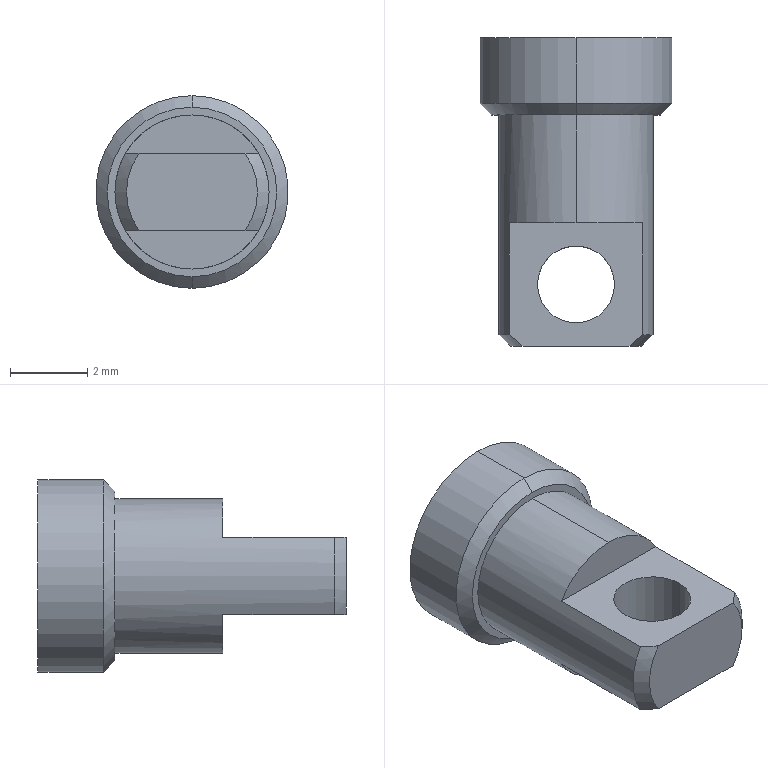Part | SolidWorks | features ICE 3, Chamfer 1, Extrusion 1, HoleWzd 1 | 1 solid | 21 faces | box 5 x 8 x 5 mm | volume 68.475 mm3 | cylinder 8 | plane 7 | cone 6 | commonest cylinder face diameters 2 x2 2.5 x2 4 x2 5 x2
STEP:
#1=CARTESIAN_POINT('',(1.,1.6,-1.));
#2=VERTEX_POINT('',#1);
#3=CARTESIAN_POINT('',(-1.,1.6,-1.));
#4=VERTEX_POINT('',#3);
#5=CARTESIAN_POINT('',(0.,1.6,-1.));
#6=DIRECTION('',(0.,0.,-1.));
#7=DIRECTION('',(1.,0.,0.));
#8=AXIS2_PLACEMENT_3D('',#5,#6,#7);
#9=CIRCLE('',#8,1.);
#10=EDGE_CURVE('',#2,#4,#9,.T.);
#11=ORIENTED_EDGE('',*,*,#10,.T.);
#12=CARTESIAN_POINT('',(-1.,1.6,1.));
#13=VERTEX_POINT('',#12);
#14=CARTESIAN_POINT('',(-1.,1.6,-5.));
#15=DIRECTION('',(0.,0.,1.));
#16=VECTOR('',#15,1000.);
#17=LINE('',#14,#16);
#18=EDGE_CURVE('',#4,#13,#17,.T.);
#19=ORIENTED_EDGE('',*,*,#18,.T.);
#20=CARTESIAN_POINT('',(1.,1.6,1.));
#21=VERTEX_POINT('',#20);
#22=CARTESIAN_POINT('',(0.,1.6,1.));
#23=DIRECTION('',(0.,0.,1.));
#24=DIRECTION('',(-1.,0.,0.));
#25=AXIS2_PLACEMENT_3D('',#22,#23,#24);
#26=CIRCLE('',#25,1.);
#27=EDGE_CURVE('',#13,#21,#26,.T.);
#28=ORIENTED_EDGE('',*,*,#27,.T.);
#29=CARTESIAN_POINT('',(1.,1.6,-5.));
#30=DIRECTION('',(0.,0.,1.));
#31=VECTOR('',#30,1000.);
#32=LINE('',#29,#31);
#33=EDGE_CURVE('',#2,#21,#32,.T.);
#34=ORIENTED_EDGE('',*,*,#33,.F.);
#35=EDGE_LOOP('',(#11,#19,#28,#34));
#36=FACE_OUTER_BOUND('',#35,.T.);
#37=CARTESIAN_POINT('',(0.,1.6,-5.));
#38=DIRECTION('',(0.,0.,1.));
#39=DIRECTION('',(1.,0.,0.));
#40=AXIS2_PLACEMENT_3D('',#37,#38,#39);
#41=CYLINDRICAL_SURFACE('',#40,1.);
#42=ADVANCED_FACE('',(#36),#41,.F.);
#43=CARTESIAN_POINT('',(0.,6.,-2.2));
#44=VERTEX_POINT('',#43);
#45=CARTESIAN_POINT('',(0.,6.,2.2));
#46=VERTEX_POINT('',#45);
#47=CARTESIAN_POINT('',(0.,6.,0.));
#48=DIRECTION('',(0.,-1.,0.));
#49=DIRECTION('',(0.,0.,1.));
#50=AXIS2_PLACEMENT_3D('',#47,#48,#49);
#51=CIRCLE('',#50,2.2);
#52=EDGE_CURVE('',#44,#46,#51,.T.);
#53=ORIENTED_EDGE('',*,*,#52,.F.);
#54=CARTESIAN_POINT('',(0.,6.3,-2.5));
#55=VERTEX_POINT('',#54);
#56=CARTESIAN_POINT('',(0.,6.3,-2.5));
#57=DIRECTION('',(0.,0.7071,-0.7071));
#58=VECTOR('',#57,1000.);
#59=LINE('',#56,#58);
#60=EDGE_CURVE('',#44,#55,#59,.T.);
#61=ORIENTED_EDGE('',*,*,#60,.T.);
#62=CARTESIAN_POINT('',(0.,6.3,2.5));
#63=VERTEX_POINT('',#62);
#64=CARTESIAN_POINT('',(0.,6.3,0.));
#65=DIRECTION('',(0.,1.,0.));
#66=DIRECTION('',(0.,0.,1.));
#67=AXIS2_PLACEMENT_3D('',#64,#65,#66);
#68=CIRCLE('',#67,2.5);
#69=EDGE_CURVE('',#63,#55,#68,.T.);
#70=ORIENTED_EDGE('',*,*,#69,.F.);
#71=CARTESIAN_POINT('',(0.,6.3,2.5));
#72=DIRECTION('',(0.,0.7071,0.7071));
#73=VECTOR('',#72,1000.);
#74=LINE('',#71,#73);
#75=EDGE_CURVE('',#46,#63,#74,.T.);
#76=ORIENTED_EDGE('',*,*,#75,.F.);
#77=EDGE_LOOP('',(#53,#61,#70,#76));
#78=FACE_OUTER_BOUND('',#77,.T.);
#79=CARTESIAN_POINT('',(0.,6.3,0.));
#80=DIRECTION('',(0.,1.,0.));
#81=DIRECTION('',(0.,0.,1.));
#82=AXIS2_PLACEMENT_3D('',#79,#80,#81);
#83=CONICAL_SURFACE('',#82,2.5,0.7854);
#84=ADVANCED_FACE('',(#78),#83,.T.);
#85=CARTESIAN_POINT('',(0.,3.5,-1.25));
#86=VERTEX_POINT('',#85);
#87=CARTESIAN_POINT('',(0.,3.5,1.25));
#88=VERTEX_POINT('',#87);
#89=CARTESIAN_POINT('',(0.,3.5,0.));
#90=DIRECTION('',(0.,1.,0.));
#91=DIRECTION('',(0.,0.,1.));
#92=AXIS2_PLACEMENT_3D('',#89,#90,#91);
#93=CIRCLE('',#92,1.25);
#94=EDGE_CURVE('',#86,#88,#93,.T.);
#95=ORIENTED_EDGE('',*,*,#94,.F.);
#96=CARTESIAN_POINT('',(0.,8.,-1.25));
#97=VERTEX_POINT('',#96);
#98=CARTESIAN_POINT('',(0.,8.,-1.25));
#99=DIRECTION('',(0.,1.,0.));
#100=VECTOR('',#99,1000.);
#101=LINE('',#98,#100);
#102=EDGE_CURVE('',#86,#97,#101,.T.);
#103=ORIENTED_EDGE('',*,*,#102,.T.);
#104=CARTESIAN_POINT('',(0.,8.,1.25));
#105=VERTEX_POINT('',#104);
#106=CARTESIAN_POINT('',(0.,8.,0.));
#107=DIRECTION('',(0.,1.,0.));
#108=DIRECTION('',(0.,0.,1.));
#109=AXIS2_PLACEMENT_3D('',#106,#107,#108);
#110=CIRCLE('',#109,1.25);
#111=EDGE_CURVE('',#97,#105,#110,.T.);
#112=ORIENTED_EDGE('',*,*,#111,.T.);
#113=CARTESIAN_POINT('',(0.,8.,1.25));
#114=DIRECTION('',(0.,1.,0.));
#115=VECTOR('',#114,1000.);
#116=LINE('',#113,#115);
#117=EDGE_CURVE('',#88,#105,#116,.T.);
#118=ORIENTED_EDGE('',*,*,#117,.F.);
#119=EDGE_LOOP('',(#95,#103,#112,#118));
#120=FACE_OUTER_BOUND('',#119,.T.);
#121=CARTESIAN_POINT('',(0.,8.,0.));
#122=DIRECTION('',(0.,1.,0.));
#123=DIRECTION('',(0.,0.,1.));
#124=AXIS2_PLACEMENT_3D('',#121,#122,#123);
#125=CYLINDRICAL_SURFACE('',#124,1.25);
#126=ADVANCED_FACE('',(#120),#125,.F.);
#127=CARTESIAN_POINT('',(0.,2.749,0.));
#128=VERTEX_POINT('',#127);
#129=CARTESIAN_POINT('',(0.,3.5,1.25));
#130=DIRECTION('',(0.,0.515,0.8572));
#131=VECTOR('',#130,1000.);
#132=LINE('',#129,#131);
#133=EDGE_CURVE('',#128,#88,#132,.T.);
#134=ORIENTED_EDGE('',*,*,#133,.F.);
#135=CARTESIAN_POINT('',(0.,3.5,-1.25));
#136=DIRECTION('',(0.,0.515,-0.8572));
#137=VECTOR('',#136,1000.);
#138=LINE('',#135,#137);
#139=EDGE_CURVE('',#128,#86,#138,.T.);
#140=ORIENTED_EDGE('',*,*,#139,.T.);
#141=ORIENTED_EDGE('',*,*,#94,.T.);
#142=EDGE_LOOP('',(#134,#140,#141));
#143=FACE_OUTER_BOUND('',#142,.T.);
#144=CARTESIAN_POINT('',(0.,3.5,0.));
#145=DIRECTION('',(0.,1.,0.));
#146=DIRECTION('',(0.,0.,1.));
#147=AXIS2_PLACEMENT_3D('',#144,#145,#146);
#148=CONICAL_SURFACE('',#147,1.25,1.03);
#149=ADVANCED_FACE('',(#143),#148,.F.);
#150=CARTESIAN_POINT('',(0.,8.,2.5));
#151=VERTEX_POINT('',#150);
#152=CARTESIAN_POINT('',(0.,8.,-2.5));
#153=VERTEX_POINT('',#152);
#154=CARTESIAN_POINT('',(0.,8.,0.));
#155=DIRECTION('',(0.,1.,0.));
#156=DIRECTION('',(0.,0.,1.));
#157=AXIS2_PLACEMENT_3D('',#154,#155,#156);
#158=CIRCLE('',#157,2.5);
#159=EDGE_CURVE('',#151,#153,#158,.T.);
#160=ORIENTED_EDGE('',*,*,#159,.F.);
#161=CARTESIAN_POINT('',(0.,8.,2.5));
#162=DIRECTION('',(0.,-1.,0.));
#163=VECTOR('',#162,1000.);
#164=LINE('',#161,#163);
#165=EDGE_CURVE('',#151,#63,#164,.T.);
#166=ORIENTED_EDGE('',*,*,#165,.T.);
#167=ORIENTED_EDGE('',*,*,#69,.T.);
#168=CARTESIAN_POINT('',(0.,8.,-2.5));
#169=DIRECTION('',(0.,-1.,0.));
#170=VECTOR('',#169,1000.);
#171=LINE('',#168,#170);
#172=EDGE_CURVE('',#153,#55,#171,.T.);
#173=ORIENTED_EDGE('',*,*,#172,.F.);
#174=EDGE_LOOP('',(#160,#166,#167,#173));
#175=FACE_OUTER_BOUND('',#174,.T.);
#176=CARTESIAN_POINT('',(0.,8.,0.));
#177=DIRECTION('',(0.,-1.,0.));
#178=DIRECTION('',(0.,0.,-1.));
#179=AXIS2_PLACEMENT_3D('',#176,#177,#178);
#180=CYLINDRICAL_SURFACE('',#179,2.5);
#181=ADVANCED_FACE('',(#175),#180,.T.);
#182=CARTESIAN_POINT('',(0.,6.,2.));
#183=VERTEX_POINT('',#182);
#184=CARTESIAN_POINT('',(0.,6.,-2.));
#185=VERTEX_POINT('',#184);
#186=CARTESIAN_POINT('',(0.,6.,0.));
#187=DIRECTION('',(0.,1.,0.));
#188=DIRECTION('',(0.,0.,1.));
#189=AXIS2_PLACEMENT_3D('',#186,#187,#188);
#190=CIRCLE('',#189,2.);
#191=EDGE_CURVE('',#183,#185,#190,.T.);
#192=ORIENTED_EDGE('',*,*,#191,.F.);
#193=CARTESIAN_POINT('',(0.,3.2,2.));
#194=VERTEX_POINT('',#193);
#195=CARTESIAN_POINT('',(0.,6.,2.));
#196=DIRECTION('',(0.,-1.,0.));
#197=VECTOR('',#196,1000.);
#198=LINE('',#195,#197);
#199=EDGE_CURVE('',#183,#194,#198,.T.);
#200=ORIENTED_EDGE('',*,*,#199,.T.);
#201=CARTESIAN_POINT('',(1.732,3.2,1.));
#202=VERTEX_POINT('',#201);
#203=CARTESIAN_POINT('',(0.,3.2,0.));
#204=DIRECTION('',(0.,1.,0.));
#205=DIRECTION('',(0.,0.,1.));
#206=AXIS2_PLACEMENT_3D('',#203,#204,#205);
#207=CIRCLE('',#206,2.);
#208=EDGE_CURVE('',#194,#202,#207,.T.);
#209=ORIENTED_EDGE('',*,*,#208,.T.);
#210=CARTESIAN_POINT('',(1.732,0.3,1.));
#211=VERTEX_POINT('',#210);
#212=CARTESIAN_POINT('',(1.732,6.,1.));
#213=DIRECTION('',(0.,-1.,0.));
#214=VECTOR('',#213,1000.);
#215=LINE('',#212,#214);
#216=EDGE_CURVE('',#202,#211,#215,.T.);
#217=ORIENTED_EDGE('',*,*,#216,.T.);
#218=CARTESIAN_POINT('',(1.732,0.3,-1.));
#219=VERTEX_POINT('',#218);
#220=CARTESIAN_POINT('',(0.,0.3,0.));
#221=DIRECTION('',(0.,1.,0.));
#222=DIRECTION('',(0.,0.,1.));
#223=AXIS2_PLACEMENT_3D('',#220,#221,#222);
#224=CIRCLE('',#223,2.);
#225=EDGE_CURVE('',#211,#219,#224,.T.);
#226=ORIENTED_EDGE('',*,*,#225,.T.);
#227=CARTESIAN_POINT('',(1.732,3.2,-1.));
#228=VERTEX_POINT('',#227);
#229=CARTESIAN_POINT('',(1.732,6.,-1.));
#230=DIRECTION('',(0.,1.,0.));
#231=VECTOR('',#230,1000.);
#232=LINE('',#229,#231);
#233=EDGE_CURVE('',#219,#228,#232,.T.);
#234=ORIENTED_EDGE('',*,*,#233,.T.);
#235=CARTESIAN_POINT('',(0.,3.2,-2.));
#236=VERTEX_POINT('',#235);
#237=CARTESIAN_POINT('',(0.,3.2,0.));
#238=DIRECTION('',(0.,1.,0.));
#239=DIRECTION('',(0.,0.,1.));
#240=AXIS2_PLACEMENT_3D('',#237,#238,#239);
#241=CIRCLE('',#240,2.);
#242=EDGE_CURVE('',#228,#236,#241,.T.);
#243=ORIENTED_EDGE('',*,*,#242,.T.);
#244=CARTESIAN_POINT('',(0.,6.,-2.));
#245=DIRECTION('',(0.,-1.,0.));
#246=VECTOR('',#245,1000.);
#247=LINE('',#244,#246);
#248=EDGE_CURVE('',#185,#236,#247,.T.);
#249=ORIENTED_EDGE('',*,*,#248,.F.);
#250=EDGE_LOOP('',(#192,#200,#209,#217,#226,#234,#243,#249));
#251=FACE_OUTER_BOUND('',#250,.T.);
#252=CARTESIAN_POINT('',(0.,6.,0.));
#253=DIRECTION('',(0.,-1.,0.));
#254=DIRECTION('',(0.,0.,-1.));
#255=AXIS2_PLACEMENT_3D('',#252,#253,#254);
#256=CYLINDRICAL_SURFACE('',#255,2.);
#257=ADVANCED_FACE('',(#251),#256,.T.);
#258=CARTESIAN_POINT('',(-1.732,0.3,1.));
#259=VERTEX_POINT('',#258);
#260=CARTESIAN_POINT('',(-1.375,0.,1.));
#261=VERTEX_POINT('',#260);
#262=CARTESIAN_POINT('',(-1.732,0.3,1.));
#263=CARTESIAN_POINT('',(-1.615,0.1982,1.));
#264=CARTESIAN_POINT('',(-1.496,0.09775,1.));
#265=CARTESIAN_POINT('',(-1.375,0.,1.));
#266=B_SPLINE_CURVE_WITH_KNOTS('',3,(#262,#263,#264,#265),.UNSPECIFIED.,.F.,.F.,(4,4),(0.003514,0.00398),.UNSPECIFIED.);
#267=EDGE_CURVE('',#259,#261,#266,.T.);
#268=ORIENTED_EDGE('',*,*,#267,.F.);
#269=CARTESIAN_POINT('',(-1.732,0.3,-1.));
#270=VERTEX_POINT('',#269);
#271=CARTESIAN_POINT('',(0.,0.3,0.));
#272=DIRECTION('',(0.,1.,0.));
#273=DIRECTION('',(0.,0.,1.));
#274=AXIS2_PLACEMENT_3D('',#271,#272,#273);
#275=CIRCLE('',#274,2.);
#276=EDGE_CURVE('',#270,#259,#275,.T.);
#277=ORIENTED_EDGE('',*,*,#276,.F.);
#278=CARTESIAN_POINT('',(-1.375,0.,-1.));
#279=VERTEX_POINT('',#278);
#280=CARTESIAN_POINT('',(-1.375,0.,-1.));
#281=CARTESIAN_POINT('',(-1.496,0.09787,-1.));
#282=CARTESIAN_POINT('',(-1.615,0.1982,-1.));
#283=CARTESIAN_POINT('',(-1.732,0.3,-1.));
#284=B_SPLINE_CURVE_WITH_KNOTS('',3,(#280,#281,#282,#283),.UNSPECIFIED.,.F.,.F.,(4,4),(0.007096,0.007558),.UNSPECIFIED.);
#285=EDGE_CURVE('',#279,#270,#284,.T.);
#286=ORIENTED_EDGE('',*,*,#285,.F.);
#287=CARTESIAN_POINT('',(0.,0.,0.));
#288=DIRECTION('',(0.,-1.,0.));
#289=DIRECTION('',(0.,0.,1.));
#290=AXIS2_PLACEMENT_3D('',#287,#288,#289);
#291=CIRCLE('',#290,1.7);
#292=EDGE_CURVE('',#261,#279,#291,.T.);
#293=ORIENTED_EDGE('',*,*,#292,.F.);
#294=EDGE_LOOP('',(#268,#277,#286,#293));
#295=FACE_OUTER_BOUND('',#294,.T.);
#296=CARTESIAN_POINT('',(0.,0.3,0.));
#297=DIRECTION('',(0.,1.,0.));
#298=DIRECTION('',(0.,0.,1.));
#299=AXIS2_PLACEMENT_3D('',#296,#297,#298);
#300=CONICAL_SURFACE('',#299,2.,0.7854);
#301=ADVANCED_FACE('',(#295),#300,.T.);
#302=ORIENTED_EDGE('',*,*,#199,.F.);
#303=CARTESIAN_POINT('',(0.,6.,0.));
#304=DIRECTION('',(0.,1.,0.));
#305=DIRECTION('',(0.,0.,1.));
#306=AXIS2_PLACEMENT_3D('',#303,#304,#305);
#307=CIRCLE('',#306,2.);
#308=EDGE_CURVE('',#185,#183,#307,.T.);
#309=ORIENTED_EDGE('',*,*,#308,.F.);
#310=ORIENTED_EDGE('',*,*,#248,.T.);
#311=CARTESIAN_POINT('',(-1.732,3.2,-1.));
#312=VERTEX_POINT('',#311);
#313=CARTESIAN_POINT('',(0.,3.2,0.));
#314=DIRECTION('',(0.,1.,0.));
#315=DIRECTION('',(0.,0.,1.));
#316=AXIS2_PLACEMENT_3D('',#313,#314,#315);
#317=CIRCLE('',#316,2.);
#318=EDGE_CURVE('',#236,#312,#317,.T.);
#319=ORIENTED_EDGE('',*,*,#318,.T.);
#320=CARTESIAN_POINT('',(-1.732,6.,-1.));
#321=DIRECTION('',(0.,-1.,0.));
#322=VECTOR('',#321,1000.);
#323=LINE('',#320,#322);
#324=EDGE_CURVE('',#312,#270,#323,.T.);
#325=ORIENTED_EDGE('',*,*,#324,.T.);
#326=ORIENTED_EDGE('',*,*,#276,.T.);
#327=CARTESIAN_POINT('',(-1.732,3.2,1.));
#328=VERTEX_POINT('',#327);
#329=CARTESIAN_POINT('',(-1.732,6.,1.));
#330=DIRECTION('',(0.,1.,0.));
#331=VECTOR('',#330,1000.);
#332=LINE('',#329,#331);
#333=EDGE_CURVE('',#259,#328,#332,.T.);
#334=ORIENTED_EDGE('',*,*,#333,.T.);
#335=CARTESIAN_POINT('',(0.,3.2,0.));
#336=DIRECTION('',(0.,1.,0.));
#337=DIRECTION('',(0.,0.,1.));
#338=AXIS2_PLACEMENT_3D('',#335,#336,#337);
#339=CIRCLE('',#338,2.);
#340=EDGE_CURVE('',#328,#194,#339,.T.);
#341=ORIENTED_EDGE('',*,*,#340,.T.);
#342=EDGE_LOOP('',(#302,#309,#310,#319,#325,#326,#334,#341));
#343=FACE_OUTER_BOUND('',#342,.T.);
#344=CARTESIAN_POINT('',(0.,6.,0.));
#345=DIRECTION('',(0.,-1.,0.));
#346=DIRECTION('',(0.,0.,-1.));
#347=AXIS2_PLACEMENT_3D('',#344,#345,#346);
#348=CYLINDRICAL_SURFACE('',#347,2.);
#349=ADVANCED_FACE('',(#343),#348,.T.);
#350=CARTESIAN_POINT('',(1.375,0.,-1.));
#351=VERTEX_POINT('',#350);
#352=CARTESIAN_POINT('',(1.375,0.,1.));
#353=VERTEX_POINT('',#352);
#354=CARTESIAN_POINT('',(0.,0.,0.));
#355=DIRECTION('',(0.,-1.,0.));
#356=DIRECTION('',(0.,0.,1.));
#357=AXIS2_PLACEMENT_3D('',#354,#355,#356);
#358=CIRCLE('',#357,1.7);
#359=EDGE_CURVE('',#351,#353,#358,.T.);
#360=ORIENTED_EDGE('',*,*,#359,.T.);
#361=CARTESIAN_POINT('',(-5.,0.,1.));
#362=DIRECTION('',(1.,0.,0.));
#363=VECTOR('',#362,1000.);
#364=LINE('',#361,#363);
#365=EDGE_CURVE('',#261,#353,#364,.T.);
#366=ORIENTED_EDGE('',*,*,#365,.F.);
#367=ORIENTED_EDGE('',*,*,#292,.T.);
#368=CARTESIAN_POINT('',(-5.,0.,-1.));
#369=DIRECTION('',(1.,0.,0.));
#370=VECTOR('',#369,1000.);
#371=LINE('',#368,#370);
#372=EDGE_CURVE('',#279,#351,#371,.T.);
#373=ORIENTED_EDGE('',*,*,#372,.T.);
#374=EDGE_LOOP('',(#360,#366,#367,#373));
#375=FACE_OUTER_BOUND('',#374,.T.);
#376=CARTESIAN_POINT('',(0.,0.,0.));
#377=DIRECTION('',(0.,1.,0.));
#378=DIRECTION('',(0.,0.,1.));
#379=AXIS2_PLACEMENT_3D('',#376,#377,#378);
#380=PLANE('',#379);
#381=ADVANCED_FACE('',(#375),#380,.F.);
#382=CARTESIAN_POINT('',(0.,6.,0.));
#383=DIRECTION('',(0.,-1.,0.));
#384=DIRECTION('',(0.,0.,1.));
#385=AXIS2_PLACEMENT_3D('',#382,#383,#384);
#386=CIRCLE('',#385,2.2);
#387=EDGE_CURVE('',#46,#44,#386,.T.);
#388=ORIENTED_EDGE('',*,*,#387,.T.);
#389=ORIENTED_EDGE('',*,*,#52,.T.);
#390=EDGE_LOOP('',(#388,#389));
#391=FACE_OUTER_BOUND('',#390,.T.);
#392=ORIENTED_EDGE('',*,*,#308,.T.);
#393=ORIENTED_EDGE('',*,*,#191,.T.);
#394=EDGE_LOOP('',(#392,#393));
#395=FACE_BOUND('',#394,.T.);
#396=CARTESIAN_POINT('',(0.,6.,0.));
#397=DIRECTION('',(0.,1.,0.));
#398=DIRECTION('',(0.,0.,1.));
#399=AXIS2_PLACEMENT_3D('',#396,#397,#398);
#400=PLANE('',#399);
#401=ADVANCED_FACE('',(#391,#395),#400,.F.);
#402=ORIENTED_EDGE('',*,*,#165,.F.);
#403=CARTESIAN_POINT('',(0.,8.,0.));
#404=DIRECTION('',(0.,1.,0.));
#405=DIRECTION('',(0.,0.,1.));
#406=AXIS2_PLACEMENT_3D('',#403,#404,#405);
#407=CIRCLE('',#406,2.5);
#408=EDGE_CURVE('',#153,#151,#407,.T.);
#409=ORIENTED_EDGE('',*,*,#408,.F.);
#410=ORIENTED_EDGE('',*,*,#172,.T.);
#411=CARTESIAN_POINT('',(0.,6.3,0.));
#412=DIRECTION('',(0.,1.,0.));
#413=DIRECTION('',(0.,0.,1.));
#414=AXIS2_PLACEMENT_3D('',#411,#412,#413);
#415=CIRCLE('',#414,2.5);
#416=EDGE_CURVE('',#55,#63,#415,.T.);
#417=ORIENTED_EDGE('',*,*,#416,.T.);
#418=EDGE_LOOP('',(#402,#409,#410,#417));
#419=FACE_OUTER_BOUND('',#418,.T.);
#420=CARTESIAN_POINT('',(0.,8.,0.));
#421=DIRECTION('',(0.,-1.,0.));
#422=DIRECTION('',(0.,0.,-1.));
#423=AXIS2_PLACEMENT_3D('',#420,#421,#422);
#424=CYLINDRICAL_SURFACE('',#423,2.5);
#425=ADVANCED_FACE('',(#419),#424,.T.);
#426=CARTESIAN_POINT('',(0.,8.,0.));
#427=DIRECTION('',(0.,1.,0.));
#428=DIRECTION('',(0.,0.,1.));
#429=AXIS2_PLACEMENT_3D('',#426,#427,#428);
#430=CIRCLE('',#429,1.25);
#431=EDGE_CURVE('',#105,#97,#430,.T.);
#432=ORIENTED_EDGE('',*,*,#431,.F.);
#433=ORIENTED_EDGE('',*,*,#111,.F.);
#434=EDGE_LOOP('',(#432,#433));
#435=FACE_BOUND('',#434,.T.);
#436=ORIENTED_EDGE('',*,*,#408,.T.);
#437=ORIENTED_EDGE('',*,*,#159,.T.);
#438=EDGE_LOOP('',(#436,#437));
#439=FACE_OUTER_BOUND('',#438,.T.);
#440=CARTESIAN_POINT('',(0.,8.,0.));
#441=DIRECTION('',(0.,1.,0.));
#442=DIRECTION('',(0.,0.,1.));
#443=AXIS2_PLACEMENT_3D('',#440,#441,#442);
#444=PLANE('',#443);
#445=ADVANCED_FACE('',(#435,#439),#444,.T.);
#446=ORIENTED_EDGE('',*,*,#139,.F.);
#447=ORIENTED_EDGE('',*,*,#133,.T.);
#448=CARTESIAN_POINT('',(0.,3.5,0.));
#449=DIRECTION('',(0.,1.,0.));
#450=DIRECTION('',(0.,0.,1.));
#451=AXIS2_PLACEMENT_3D('',#448,#449,#450);
#452=CIRCLE('',#451,1.25);
#453=EDGE_CURVE('',#88,#86,#452,.T.);
#454=ORIENTED_EDGE('',*,*,#453,.T.);
#455=EDGE_LOOP('',(#446,#447,#454));
#456=FACE_OUTER_BOUND('',#455,.T.);
#457=CARTESIAN_POINT('',(0.,3.5,0.));
#458=DIRECTION('',(0.,1.,0.));
#459=DIRECTION('',(0.,0.,1.));
#460=AXIS2_PLACEMENT_3D('',#457,#458,#459);
#461=CONICAL_SURFACE('',#460,1.25,1.03);
#462=ADVANCED_FACE('',(#456),#461,.F.);
#463=ORIENTED_EDGE('',*,*,#102,.F.);
#464=ORIENTED_EDGE('',*,*,#453,.F.);
#465=ORIENTED_EDGE('',*,*,#117,.T.);
#466=ORIENTED_EDGE('',*,*,#431,.T.);
#467=EDGE_LOOP('',(#463,#464,#465,#466));
#468=FACE_OUTER_BOUND('',#467,.T.);
#469=CARTESIAN_POINT('',(0.,8.,0.));
#470=DIRECTION('',(0.,1.,0.));
#471=DIRECTION('',(0.,0.,1.));
#472=AXIS2_PLACEMENT_3D('',#469,#470,#471);
#473=CYLINDRICAL_SURFACE('',#472,1.25);
#474=ADVANCED_FACE('',(#468),#473,.F.);
#475=CARTESIAN_POINT('',(1.375,0.,1.));
#476=CARTESIAN_POINT('',(1.496,0.09787,1.));
#477=CARTESIAN_POINT('',(1.615,0.1982,1.));
#478=CARTESIAN_POINT('',(1.732,0.3,1.));
#479=B_SPLINE_CURVE_WITH_KNOTS('',3,(#475,#476,#477,#478),.UNSPECIFIED.,.F.,.F.,(4,4),(0.007096,0.007558),.UNSPECIFIED.);
#480=EDGE_CURVE('',#353,#211,#479,.T.);
#481=ORIENTED_EDGE('',*,*,#480,.F.);
#482=ORIENTED_EDGE('',*,*,#359,.F.);
#483=CARTESIAN_POINT('',(1.732,0.3,-1.));
#484=CARTESIAN_POINT('',(1.615,0.1982,-1.));
#485=CARTESIAN_POINT('',(1.496,0.09775,-1.));
#486=CARTESIAN_POINT('',(1.375,0.,-1.));
#487=B_SPLINE_CURVE_WITH_KNOTS('',3,(#483,#484,#485,#486),.UNSPECIFIED.,.F.,.F.,(4,4),(0.003514,0.00398),.UNSPECIFIED.);
#488=EDGE_CURVE('',#219,#351,#487,.T.);
#489=ORIENTED_EDGE('',*,*,#488,.F.);
#490=ORIENTED_EDGE('',*,*,#225,.F.);
#491=EDGE_LOOP('',(#481,#482,#489,#490));
#492=FACE_OUTER_BOUND('',#491,.T.);
#493=CARTESIAN_POINT('',(0.,0.3,0.));
#494=DIRECTION('',(0.,1.,0.));
#495=DIRECTION('',(0.,0.,1.));
#496=AXIS2_PLACEMENT_3D('',#493,#494,#495);
#497=CONICAL_SURFACE('',#496,2.,0.7854);
#498=ADVANCED_FACE('',(#492),#497,.T.);
#499=ORIENTED_EDGE('',*,*,#60,.F.);
#500=ORIENTED_EDGE('',*,*,#387,.F.);
#501=ORIENTED_EDGE('',*,*,#75,.T.);
#502=ORIENTED_EDGE('',*,*,#416,.F.);
#503=EDGE_LOOP('',(#499,#500,#501,#502));
#504=FACE_OUTER_BOUND('',#503,.T.);
#505=CARTESIAN_POINT('',(0.,6.3,0.));
#506=DIRECTION('',(0.,1.,0.));
#507=DIRECTION('',(0.,0.,1.));
#508=AXIS2_PLACEMENT_3D('',#505,#506,#507);
#509=CONICAL_SURFACE('',#508,2.5,0.7854);
#510=ADVANCED_FACE('',(#504),#509,.T.);
#511=ORIENTED_EDGE('',*,*,#18,.F.);
#512=CARTESIAN_POINT('',(0.,1.6,-1.));
#513=DIRECTION('',(0.,0.,-1.));
#514=DIRECTION('',(1.,0.,0.));
#515=AXIS2_PLACEMENT_3D('',#512,#513,#514);
#516=CIRCLE('',#515,1.);
#517=EDGE_CURVE('',#4,#2,#516,.T.);
#518=ORIENTED_EDGE('',*,*,#517,.T.);
#519=ORIENTED_EDGE('',*,*,#33,.T.);
#520=CARTESIAN_POINT('',(0.,1.6,1.));
#521=DIRECTION('',(0.,0.,1.));
#522=DIRECTION('',(-1.,0.,0.));
#523=AXIS2_PLACEMENT_3D('',#520,#521,#522);
#524=CIRCLE('',#523,1.);
#525=EDGE_CURVE('',#21,#13,#524,.T.);
#526=ORIENTED_EDGE('',*,*,#525,.T.);
#527=EDGE_LOOP('',(#511,#518,#519,#526));
#528=FACE_OUTER_BOUND('',#527,.T.);
#529=CARTESIAN_POINT('',(0.,1.6,-5.));
#530=DIRECTION('',(0.,0.,1.));
#531=DIRECTION('',(1.,0.,0.));
#532=AXIS2_PLACEMENT_3D('',#529,#530,#531);
#533=CYLINDRICAL_SURFACE('',#532,1.);
#534=ADVANCED_FACE('',(#528),#533,.F.);
#535=CARTESIAN_POINT('',(-5.,3.2,-1.));
#536=DIRECTION('',(1.,0.,0.));
#537=VECTOR('',#536,1000.);
#538=LINE('',#535,#537);
#539=EDGE_CURVE('',#312,#228,#538,.T.);
#540=ORIENTED_EDGE('',*,*,#539,.F.);
#541=ORIENTED_EDGE('',*,*,#318,.F.);
#542=ORIENTED_EDGE('',*,*,#242,.F.);
#543=EDGE_LOOP('',(#540,#541,#542));
#544=FACE_OUTER_BOUND('',#543,.T.);
#545=CARTESIAN_POINT('',(-5.,3.2,-4.));
#546=DIRECTION('',(0.,1.,0.));
#547=DIRECTION('',(0.,0.,1.));
#548=AXIS2_PLACEMENT_3D('',#545,#546,#547);
#549=PLANE('',#548);
#550=ADVANCED_FACE('',(#544),#549,.F.);
#551=ORIENTED_EDGE('',*,*,#10,.F.);
#552=ORIENTED_EDGE('',*,*,#517,.F.);
#553=EDGE_LOOP('',(#551,#552));
#554=FACE_BOUND('',#553,.T.);
#555=ORIENTED_EDGE('',*,*,#488,.T.);
#556=ORIENTED_EDGE('',*,*,#372,.F.);
#557=ORIENTED_EDGE('',*,*,#285,.T.);
#558=ORIENTED_EDGE('',*,*,#324,.F.);
#559=ORIENTED_EDGE('',*,*,#539,.T.);
#560=ORIENTED_EDGE('',*,*,#233,.F.);
#561=EDGE_LOOP('',(#555,#556,#557,#558,#559,#560));
#562=FACE_OUTER_BOUND('',#561,.T.);
#563=CARTESIAN_POINT('',(-5.,0.,-1.));
#564=DIRECTION('',(0.,0.,1.));
#565=DIRECTION('',(1.,0.,0.));
#566=AXIS2_PLACEMENT_3D('',#563,#564,#565);
#567=PLANE('',#566);
#568=ADVANCED_FACE('',(#554,#562),#567,.F.);
#569=CARTESIAN_POINT('',(-5.,3.2,1.));
#570=DIRECTION('',(1.,0.,0.));
#571=VECTOR('',#570,1000.);
#572=LINE('',#569,#571);
#573=EDGE_CURVE('',#328,#202,#572,.T.);
#574=ORIENTED_EDGE('',*,*,#573,.T.);
#575=ORIENTED_EDGE('',*,*,#208,.F.);
#576=ORIENTED_EDGE('',*,*,#340,.F.);
#577=EDGE_LOOP('',(#574,#575,#576));
#578=FACE_OUTER_BOUND('',#577,.T.);
#579=CARTESIAN_POINT('',(-5.,3.2,4.));
#580=DIRECTION('',(0.,1.,0.));
#581=DIRECTION('',(0.,0.,1.));
#582=AXIS2_PLACEMENT_3D('',#579,#580,#581);
#583=PLANE('',#582);
#584=ADVANCED_FACE('',(#578),#583,.F.);
#585=ORIENTED_EDGE('',*,*,#525,.F.);
#586=ORIENTED_EDGE('',*,*,#27,.F.);
#587=EDGE_LOOP('',(#585,#586));
#588=FACE_BOUND('',#587,.T.);
#589=ORIENTED_EDGE('',*,*,#267,.T.);
#590=ORIENTED_EDGE('',*,*,#365,.T.);
#591=ORIENTED_EDGE('',*,*,#480,.T.);
#592=ORIENTED_EDGE('',*,*,#216,.F.);
#593=ORIENTED_EDGE('',*,*,#573,.F.);
#594=ORIENTED_EDGE('',*,*,#333,.F.);
#595=EDGE_LOOP('',(#589,#590,#591,#592,#593,#594));
#596=FACE_OUTER_BOUND('',#595,.T.);
#597=CARTESIAN_POINT('',(-5.,0.,1.));
#598=DIRECTION('',(0.,0.,-1.));
#599=DIRECTION('',(-1.,0.,0.));
#600=AXIS2_PLACEMENT_3D('',#597,#598,#599);
#601=PLANE('',#600);
#602=ADVANCED_FACE('',(#588,#596),#601,.F.);
#603=CLOSED_SHELL('',(#42,#84,#126,#149,#181,#257,#301,#349,#381,#401,#425,#445,#462,#474,#498,#510,#534,#550,#568,#584,#602));
#604=MANIFOLD_SOLID_BREP('',#603);
#605=CARTESIAN_POINT('',(0.,0.,0.));
#606=DIRECTION('',(0.,0.,1.));
#607=DIRECTION('',(1.,0.,0.));
#608=AXIS2_PLACEMENT_3D('',#605,#606,#607);
#609=(LENGTH_UNIT()NAMED_UNIT(*)SI_UNIT(.MILLI.,.METRE.));
#610=UNCERTAINTY_MEASURE_WITH_UNIT(LENGTH_MEASURE(0.00001),#609,'','');
#611=(NAMED_UNIT(*)PLANE_ANGLE_UNIT()SI_UNIT($,.RADIAN.));
#612=(NAMED_UNIT(*)SI_UNIT($,.STERADIAN.)SOLID_ANGLE_UNIT());
#613=(GEOMETRIC_REPRESENTATION_CONTEXT(3)GLOBAL_UNCERTAINTY_ASSIGNED_CONTEXT((#610))GLOBAL_UNIT_ASSIGNED_CONTEXT((#609,#611,#612))REPRESENTATION_CONTEXT('',''));
#614=ADVANCED_BREP_SHAPE_REPRESENTATION('',(#604,#608),#613);